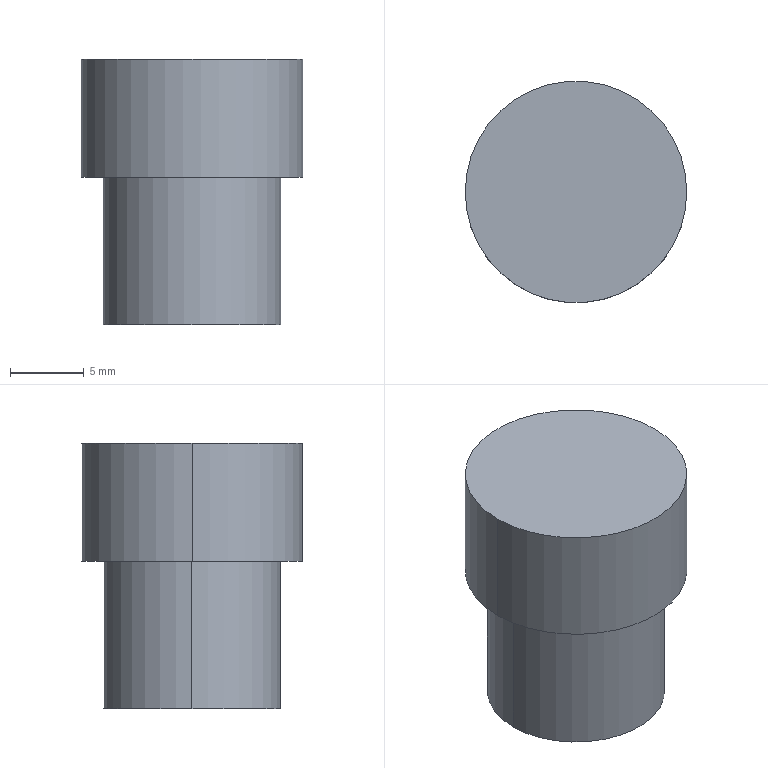Part | SolidWorks | features Extrusion 1, ICE 1 | 1 solid | 7 faces | box 15 x 15 x 18 mm | volume 2545 mm3 | cylinder 4 | plane 3 | commonest cylinder face diameters 12 x2 15 x2
STEP:
#1=CARTESIAN_POINT('',(7.5,0.,8.));
#2=VERTEX_POINT('',#1);
#3=CARTESIAN_POINT('',(-7.5,0.,8.));
#4=VERTEX_POINT('',#3);
#5=CARTESIAN_POINT('',(0.,0.,8.));
#6=DIRECTION('',(0.,0.,1.));
#7=DIRECTION('',(1.,0.,0.));
#8=AXIS2_PLACEMENT_3D('',#5,#6,#7);
#9=CIRCLE('',#8,7.5);
#10=EDGE_CURVE('',#2,#4,#9,.T.);
#11=ORIENTED_EDGE('',*,*,#10,.F.);
#12=CARTESIAN_POINT('',(7.5,0.,0.));
#13=VERTEX_POINT('',#12);
#14=CARTESIAN_POINT('',(7.5,0.,8.));
#15=DIRECTION('',(0.,0.,-1.));
#16=VECTOR('',#15,1000.);
#17=LINE('',#14,#16);
#18=EDGE_CURVE('',#2,#13,#17,.T.);
#19=ORIENTED_EDGE('',*,*,#18,.T.);
#20=CARTESIAN_POINT('',(-7.5,0.,0.));
#21=VERTEX_POINT('',#20);
#22=CARTESIAN_POINT('',(0.,0.,0.));
#23=DIRECTION('',(0.,0.,1.));
#24=DIRECTION('',(1.,0.,0.));
#25=AXIS2_PLACEMENT_3D('',#22,#23,#24);
#26=CIRCLE('',#25,7.5);
#27=EDGE_CURVE('',#13,#21,#26,.T.);
#28=ORIENTED_EDGE('',*,*,#27,.T.);
#29=CARTESIAN_POINT('',(-7.5,0.,8.));
#30=DIRECTION('',(0.,0.,-1.));
#31=VECTOR('',#30,1000.);
#32=LINE('',#29,#31);
#33=EDGE_CURVE('',#4,#21,#32,.T.);
#34=ORIENTED_EDGE('',*,*,#33,.F.);
#35=EDGE_LOOP('',(#11,#19,#28,#34));
#36=FACE_OUTER_BOUND('',#35,.T.);
#37=CARTESIAN_POINT('',(0.,0.,8.));
#38=DIRECTION('',(0.,0.,-1.));
#39=DIRECTION('',(-1.,0.,0.));
#40=AXIS2_PLACEMENT_3D('',#37,#38,#39);
#41=CYLINDRICAL_SURFACE('',#40,7.5);
#42=ADVANCED_FACE('',(#36),#41,.T.);
#43=CARTESIAN_POINT('',(6.,0.,-10.));
#44=VERTEX_POINT('',#43);
#45=CARTESIAN_POINT('',(-6.,0.,-10.));
#46=VERTEX_POINT('',#45);
#47=CARTESIAN_POINT('',(0.,0.,-10.));
#48=DIRECTION('',(0.,0.,1.));
#49=DIRECTION('',(1.,0.,0.));
#50=AXIS2_PLACEMENT_3D('',#47,#48,#49);
#51=CIRCLE('',#50,6.);
#52=EDGE_CURVE('',#44,#46,#51,.T.);
#53=ORIENTED_EDGE('',*,*,#52,.T.);
#54=CARTESIAN_POINT('',(-6.,0.,0.));
#55=VERTEX_POINT('',#54);
#56=CARTESIAN_POINT('',(-6.,0.,-10.));
#57=DIRECTION('',(0.,0.,1.));
#58=VECTOR('',#57,1000.);
#59=LINE('',#56,#58);
#60=EDGE_CURVE('',#46,#55,#59,.T.);
#61=ORIENTED_EDGE('',*,*,#60,.T.);
#62=CARTESIAN_POINT('',(6.,0.,0.));
#63=VERTEX_POINT('',#62);
#64=CARTESIAN_POINT('',(0.,0.,0.));
#65=DIRECTION('',(0.,0.,1.));
#66=DIRECTION('',(1.,0.,0.));
#67=AXIS2_PLACEMENT_3D('',#64,#65,#66);
#68=CIRCLE('',#67,6.);
#69=EDGE_CURVE('',#63,#55,#68,.T.);
#70=ORIENTED_EDGE('',*,*,#69,.F.);
#71=CARTESIAN_POINT('',(6.,0.,-10.));
#72=DIRECTION('',(0.,0.,1.));
#73=VECTOR('',#72,1000.);
#74=LINE('',#71,#73);
#75=EDGE_CURVE('',#44,#63,#74,.T.);
#76=ORIENTED_EDGE('',*,*,#75,.F.);
#77=EDGE_LOOP('',(#53,#61,#70,#76));
#78=FACE_OUTER_BOUND('',#77,.T.);
#79=CARTESIAN_POINT('',(0.,0.,-10.));
#80=DIRECTION('',(0.,0.,1.));
#81=DIRECTION('',(1.,0.,0.));
#82=AXIS2_PLACEMENT_3D('',#79,#80,#81);
#83=CYLINDRICAL_SURFACE('',#82,6.);
#84=ADVANCED_FACE('',(#78),#83,.T.);
#85=ORIENTED_EDGE('',*,*,#60,.F.);
#86=CARTESIAN_POINT('',(0.,0.,-10.));
#87=DIRECTION('',(0.,0.,1.));
#88=DIRECTION('',(1.,0.,0.));
#89=AXIS2_PLACEMENT_3D('',#86,#87,#88);
#90=CIRCLE('',#89,6.);
#91=EDGE_CURVE('',#46,#44,#90,.T.);
#92=ORIENTED_EDGE('',*,*,#91,.T.);
#93=ORIENTED_EDGE('',*,*,#75,.T.);
#94=CARTESIAN_POINT('',(0.,0.,0.));
#95=DIRECTION('',(0.,0.,1.));
#96=DIRECTION('',(1.,0.,0.));
#97=AXIS2_PLACEMENT_3D('',#94,#95,#96);
#98=CIRCLE('',#97,6.);
#99=EDGE_CURVE('',#55,#63,#98,.T.);
#100=ORIENTED_EDGE('',*,*,#99,.F.);
#101=EDGE_LOOP('',(#85,#92,#93,#100));
#102=FACE_OUTER_BOUND('',#101,.T.);
#103=CARTESIAN_POINT('',(0.,0.,-10.));
#104=DIRECTION('',(0.,0.,1.));
#105=DIRECTION('',(1.,0.,0.));
#106=AXIS2_PLACEMENT_3D('',#103,#104,#105);
#107=CYLINDRICAL_SURFACE('',#106,6.);
#108=ADVANCED_FACE('',(#102),#107,.T.);
#109=ORIENTED_EDGE('',*,*,#52,.F.);
#110=ORIENTED_EDGE('',*,*,#91,.F.);
#111=EDGE_LOOP('',(#109,#110));
#112=FACE_OUTER_BOUND('',#111,.T.);
#113=CARTESIAN_POINT('',(0.,0.,-10.));
#114=DIRECTION('',(0.,0.,1.));
#115=DIRECTION('',(1.,0.,0.));
#116=AXIS2_PLACEMENT_3D('',#113,#114,#115);
#117=PLANE('',#116);
#118=ADVANCED_FACE('',(#112),#117,.F.);
#119=ORIENTED_EDGE('',*,*,#18,.F.);
#120=CARTESIAN_POINT('',(0.,0.,8.));
#121=DIRECTION('',(0.,0.,1.));
#122=DIRECTION('',(1.,0.,0.));
#123=AXIS2_PLACEMENT_3D('',#120,#121,#122);
#124=CIRCLE('',#123,7.5);
#125=EDGE_CURVE('',#4,#2,#124,.T.);
#126=ORIENTED_EDGE('',*,*,#125,.F.);
#127=ORIENTED_EDGE('',*,*,#33,.T.);
#128=CARTESIAN_POINT('',(0.,0.,0.));
#129=DIRECTION('',(0.,0.,1.));
#130=DIRECTION('',(1.,0.,0.));
#131=AXIS2_PLACEMENT_3D('',#128,#129,#130);
#132=CIRCLE('',#131,7.5);
#133=EDGE_CURVE('',#21,#13,#132,.T.);
#134=ORIENTED_EDGE('',*,*,#133,.T.);
#135=EDGE_LOOP('',(#119,#126,#127,#134));
#136=FACE_OUTER_BOUND('',#135,.T.);
#137=CARTESIAN_POINT('',(0.,0.,8.));
#138=DIRECTION('',(0.,0.,-1.));
#139=DIRECTION('',(-1.,0.,0.));
#140=AXIS2_PLACEMENT_3D('',#137,#138,#139);
#141=CYLINDRICAL_SURFACE('',#140,7.5);
#142=ADVANCED_FACE('',(#136),#141,.T.);
#143=ORIENTED_EDGE('',*,*,#125,.T.);
#144=ORIENTED_EDGE('',*,*,#10,.T.);
#145=EDGE_LOOP('',(#143,#144));
#146=FACE_OUTER_BOUND('',#145,.T.);
#147=CARTESIAN_POINT('',(0.,0.,8.));
#148=DIRECTION('',(0.,0.,1.));
#149=DIRECTION('',(1.,0.,0.));
#150=AXIS2_PLACEMENT_3D('',#147,#148,#149);
#151=PLANE('',#150);
#152=ADVANCED_FACE('',(#146),#151,.T.);
#153=ORIENTED_EDGE('',*,*,#69,.T.);
#154=ORIENTED_EDGE('',*,*,#99,.T.);
#155=EDGE_LOOP('',(#153,#154));
#156=FACE_BOUND('',#155,.T.);
#157=ORIENTED_EDGE('',*,*,#133,.F.);
#158=ORIENTED_EDGE('',*,*,#27,.F.);
#159=EDGE_LOOP('',(#157,#158));
#160=FACE_OUTER_BOUND('',#159,.T.);
#161=CARTESIAN_POINT('',(0.,0.,0.));
#162=DIRECTION('',(0.,0.,1.));
#163=DIRECTION('',(1.,0.,0.));
#164=AXIS2_PLACEMENT_3D('',#161,#162,#163);
#165=PLANE('',#164);
#166=ADVANCED_FACE('',(#156,#160),#165,.F.);
#167=CLOSED_SHELL('',(#42,#84,#108,#118,#142,#152,#166));
#168=MANIFOLD_SOLID_BREP('',#167);
#169=CARTESIAN_POINT('',(0.,0.,0.));
#170=DIRECTION('',(0.,0.,1.));
#171=DIRECTION('',(1.,0.,0.));
#172=AXIS2_PLACEMENT_3D('',#169,#170,#171);
#173=(LENGTH_UNIT()NAMED_UNIT(*)SI_UNIT(.MILLI.,.METRE.));
#174=UNCERTAINTY_MEASURE_WITH_UNIT(LENGTH_MEASURE(0.00001),#173,'','');
#175=(NAMED_UNIT(*)PLANE_ANGLE_UNIT()SI_UNIT($,.RADIAN.));
#176=(NAMED_UNIT(*)SI_UNIT($,.STERADIAN.)SOLID_ANGLE_UNIT());
#177=(GEOMETRIC_REPRESENTATION_CONTEXT(3)GLOBAL_UNCERTAINTY_ASSIGNED_CONTEXT((#174))GLOBAL_UNIT_ASSIGNED_CONTEXT((#173,#175,#176))REPRESENTATION_CONTEXT('',''));
#178=ADVANCED_BREP_SHAPE_REPRESENTATION('',(#168,#172),#177);